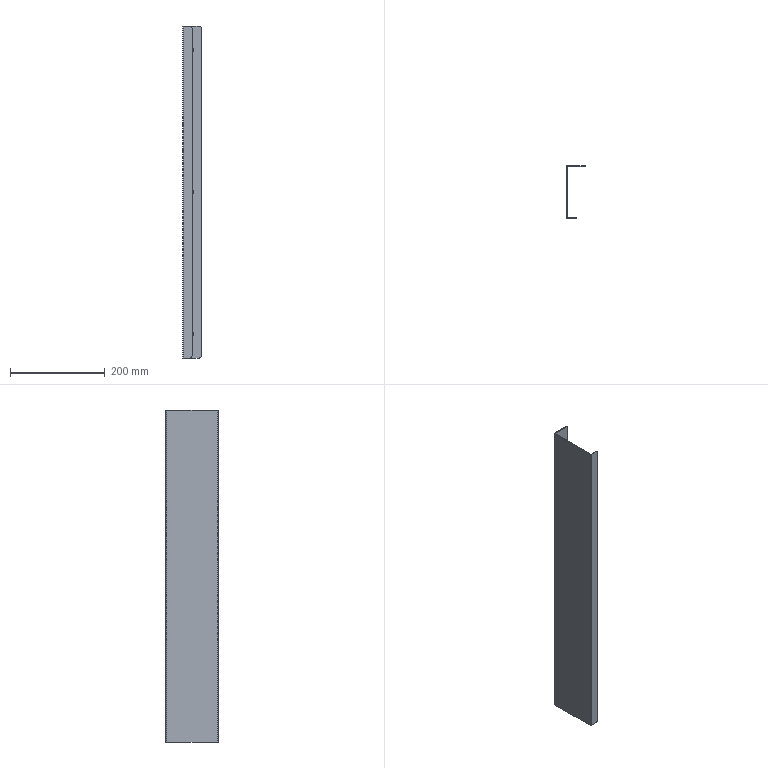Part | STEP file | HJDX-300 | 1 solid | 24 faces | box 40 x 110 x 700 mm | volume 173965 mm3 | cylinder 14 | plane 10 | commonest cylinder face diameters 8 x6 10 x4 1 x2 4 x2
STEP:
#1=CARTESIAN_POINT('',(22.5,53.5,-300.));
#2=VERTEX_POINT('',#1);
#3=CARTESIAN_POINT('',(14.5,53.5,-300.));
#4=VERTEX_POINT('',#3);
#5=CARTESIAN_POINT('',(18.5,53.5,-300.));
#6=DIRECTION('',(0.,1.,0.));
#7=DIRECTION('',(-1.,0.,0.));
#8=AXIS2_PLACEMENT_3D('',#5,#6,#7);
#9=CIRCLE('',#8,4.);
#10=EDGE_CURVE('',#2,#4,#9,.T.);
#11=ORIENTED_EDGE('',*,*,#10,.F.);
#12=CARTESIAN_POINT('',(22.5,55.,-300.));
#13=VERTEX_POINT('',#12);
#14=CARTESIAN_POINT('',(22.5,45.,-300.));
#15=DIRECTION('',(0.,1.,0.));
#16=VECTOR('',#15,1000.);
#17=LINE('',#14,#16);
#18=EDGE_CURVE('',#2,#13,#17,.T.);
#19=ORIENTED_EDGE('',*,*,#18,.T.);
#20=CARTESIAN_POINT('',(14.5,55.,-300.));
#21=VERTEX_POINT('',#20);
#22=CARTESIAN_POINT('',(18.5,55.,-300.));
#23=DIRECTION('',(0.,1.,0.));
#24=DIRECTION('',(-1.,0.,0.));
#25=AXIS2_PLACEMENT_3D('',#22,#23,#24);
#26=CIRCLE('',#25,4.);
#27=EDGE_CURVE('',#13,#21,#26,.T.);
#28=ORIENTED_EDGE('',*,*,#27,.T.);
#29=CARTESIAN_POINT('',(14.5,45.,-300.));
#30=DIRECTION('',(0.,1.,0.));
#31=VECTOR('',#30,1000.);
#32=LINE('',#29,#31);
#33=EDGE_CURVE('',#4,#21,#32,.T.);
#34=ORIENTED_EDGE('',*,*,#33,.F.);
#35=EDGE_LOOP('',(#11,#19,#28,#34));
#36=FACE_OUTER_BOUND('',#35,.T.);
#37=CARTESIAN_POINT('',(18.5,45.,-300.));
#38=DIRECTION('',(0.,1.,0.));
#39=DIRECTION('',(-1.,0.,0.));
#40=AXIS2_PLACEMENT_3D('',#37,#38,#39);
#41=CYLINDRICAL_SURFACE('',#40,4.);
#42=ADVANCED_FACE('',(#36),#41,.F.);
#43=CARTESIAN_POINT('',(22.5,53.5,300.));
#44=VERTEX_POINT('',#43);
#45=CARTESIAN_POINT('',(14.5,53.5,300.));
#46=VERTEX_POINT('',#45);
#47=CARTESIAN_POINT('',(18.5,53.5,300.));
#48=DIRECTION('',(0.,1.,0.));
#49=DIRECTION('',(-1.,0.,0.));
#50=AXIS2_PLACEMENT_3D('',#47,#48,#49);
#51=CIRCLE('',#50,4.);
#52=EDGE_CURVE('',#44,#46,#51,.T.);
#53=ORIENTED_EDGE('',*,*,#52,.F.);
#54=CARTESIAN_POINT('',(22.5,55.,300.));
#55=VERTEX_POINT('',#54);
#56=CARTESIAN_POINT('',(22.5,45.,300.));
#57=DIRECTION('',(0.,1.,0.));
#58=VECTOR('',#57,1000.);
#59=LINE('',#56,#58);
#60=EDGE_CURVE('',#44,#55,#59,.T.);
#61=ORIENTED_EDGE('',*,*,#60,.T.);
#62=CARTESIAN_POINT('',(14.5,55.,300.));
#63=VERTEX_POINT('',#62);
#64=CARTESIAN_POINT('',(18.5,55.,300.));
#65=DIRECTION('',(0.,1.,0.));
#66=DIRECTION('',(-1.,0.,0.));
#67=AXIS2_PLACEMENT_3D('',#64,#65,#66);
#68=CIRCLE('',#67,4.);
#69=EDGE_CURVE('',#55,#63,#68,.T.);
#70=ORIENTED_EDGE('',*,*,#69,.T.);
#71=CARTESIAN_POINT('',(14.5,45.,300.));
#72=DIRECTION('',(0.,1.,0.));
#73=VECTOR('',#72,1000.);
#74=LINE('',#71,#73);
#75=EDGE_CURVE('',#46,#63,#74,.T.);
#76=ORIENTED_EDGE('',*,*,#75,.F.);
#77=EDGE_LOOP('',(#53,#61,#70,#76));
#78=FACE_OUTER_BOUND('',#77,.T.);
#79=CARTESIAN_POINT('',(18.5,45.,300.));
#80=DIRECTION('',(0.,1.,0.));
#81=DIRECTION('',(-1.,0.,0.));
#82=AXIS2_PLACEMENT_3D('',#79,#80,#81);
#83=CYLINDRICAL_SURFACE('',#82,4.);
#84=ADVANCED_FACE('',(#78),#83,.F.);
#85=CARTESIAN_POINT('',(22.5,53.5,0.));
#86=VERTEX_POINT('',#85);
#87=CARTESIAN_POINT('',(14.5,53.5,0.));
#88=VERTEX_POINT('',#87);
#89=CARTESIAN_POINT('',(18.5,53.5,0.));
#90=DIRECTION('',(0.,1.,0.));
#91=DIRECTION('',(-1.,0.,0.));
#92=AXIS2_PLACEMENT_3D('',#89,#90,#91);
#93=CIRCLE('',#92,4.);
#94=EDGE_CURVE('',#86,#88,#93,.T.);
#95=ORIENTED_EDGE('',*,*,#94,.F.);
#96=CARTESIAN_POINT('',(22.5,55.,0.));
#97=VERTEX_POINT('',#96);
#98=CARTESIAN_POINT('',(22.5,45.,0.));
#99=DIRECTION('',(0.,1.,0.));
#100=VECTOR('',#99,1000.);
#101=LINE('',#98,#100);
#102=EDGE_CURVE('',#86,#97,#101,.T.);
#103=ORIENTED_EDGE('',*,*,#102,.T.);
#104=CARTESIAN_POINT('',(14.5,55.,0.));
#105=VERTEX_POINT('',#104);
#106=CARTESIAN_POINT('',(18.5,55.,0.));
#107=DIRECTION('',(0.,1.,0.));
#108=DIRECTION('',(-1.,0.,0.));
#109=AXIS2_PLACEMENT_3D('',#106,#107,#108);
#110=CIRCLE('',#109,4.);
#111=EDGE_CURVE('',#97,#105,#110,.T.);
#112=ORIENTED_EDGE('',*,*,#111,.T.);
#113=CARTESIAN_POINT('',(14.5,45.,0.));
#114=DIRECTION('',(0.,1.,0.));
#115=VECTOR('',#114,1000.);
#116=LINE('',#113,#115);
#117=EDGE_CURVE('',#88,#105,#116,.T.);
#118=ORIENTED_EDGE('',*,*,#117,.F.);
#119=EDGE_LOOP('',(#95,#103,#112,#118));
#120=FACE_OUTER_BOUND('',#119,.T.);
#121=CARTESIAN_POINT('',(18.5,45.,0.));
#122=DIRECTION('',(0.,1.,0.));
#123=DIRECTION('',(-1.,0.,0.));
#124=AXIS2_PLACEMENT_3D('',#121,#122,#123);
#125=CYLINDRICAL_SURFACE('',#124,4.);
#126=ADVANCED_FACE('',(#120),#125,.F.);
#127=CARTESIAN_POINT('',(-1.5,-53.,350.));
#128=VERTEX_POINT('',#127);
#129=CARTESIAN_POINT('',(-1.5,53.,350.));
#130=VERTEX_POINT('',#129);
#131=CARTESIAN_POINT('',(-1.5,0.,350.));
#132=DIRECTION('',(0.,1.,0.));
#133=VECTOR('',#132,1000.);
#134=LINE('',#131,#133);
#135=EDGE_CURVE('',#128,#130,#134,.T.);
#136=ORIENTED_EDGE('',*,*,#135,.T.);
#137=CARTESIAN_POINT('',(-1.5,53.,-350.));
#138=VERTEX_POINT('',#137);
#139=CARTESIAN_POINT('',(-1.5,53.,0.));
#140=DIRECTION('',(0.,0.,-1.));
#141=VECTOR('',#140,1000.);
#142=LINE('',#139,#141);
#143=EDGE_CURVE('',#130,#138,#142,.T.);
#144=ORIENTED_EDGE('',*,*,#143,.T.);
#145=CARTESIAN_POINT('',(-1.5,-53.,-350.));
#146=VERTEX_POINT('',#145);
#147=CARTESIAN_POINT('',(-1.5,0.,-350.));
#148=DIRECTION('',(0.,-1.,0.));
#149=VECTOR('',#148,1000.);
#150=LINE('',#147,#149);
#151=EDGE_CURVE('',#138,#146,#150,.T.);
#152=ORIENTED_EDGE('',*,*,#151,.T.);
#153=CARTESIAN_POINT('',(-1.5,-53.,0.));
#154=DIRECTION('',(0.,0.,1.));
#155=VECTOR('',#154,1000.);
#156=LINE('',#153,#155);
#157=EDGE_CURVE('',#146,#128,#156,.T.);
#158=ORIENTED_EDGE('',*,*,#157,.T.);
#159=EDGE_LOOP('',(#136,#144,#152,#158));
#160=FACE_OUTER_BOUND('',#159,.T.);
#161=CARTESIAN_POINT('',(-1.5,0.,0.));
#162=DIRECTION('',(-1.,0.,0.));
#163=DIRECTION('',(0.,0.,1.));
#164=AXIS2_PLACEMENT_3D('',#161,#162,#163);
#165=PLANE('',#164);
#166=ADVANCED_FACE('',(#160),#165,.T.);
#167=CARTESIAN_POINT('',(0.5,55.,350.));
#168=VERTEX_POINT('',#167);
#169=CARTESIAN_POINT('',(0.5,55.,-350.));
#170=VERTEX_POINT('',#169);
#171=CARTESIAN_POINT('',(0.5,55.,350.));
#172=DIRECTION('',(0.,0.,-1.));
#173=VECTOR('',#172,1000.);
#174=LINE('',#171,#173);
#175=EDGE_CURVE('',#168,#170,#174,.T.);
#176=ORIENTED_EDGE('',*,*,#175,.T.);
#177=CARTESIAN_POINT('',(0.5,53.,-350.));
#178=DIRECTION('',(0.,0.,1.));
#179=DIRECTION('',(1.,0.,0.));
#180=AXIS2_PLACEMENT_3D('',#177,#178,#179);
#181=CIRCLE('',#180,2.);
#182=EDGE_CURVE('',#170,#138,#181,.T.);
#183=ORIENTED_EDGE('',*,*,#182,.T.);
#184=ORIENTED_EDGE('',*,*,#143,.F.);
#185=CARTESIAN_POINT('',(0.5,53.,350.));
#186=DIRECTION('',(0.,0.,-1.));
#187=DIRECTION('',(1.,0.,0.));
#188=AXIS2_PLACEMENT_3D('',#185,#186,#187);
#189=CIRCLE('',#188,2.);
#190=EDGE_CURVE('',#130,#168,#189,.T.);
#191=ORIENTED_EDGE('',*,*,#190,.T.);
#192=EDGE_LOOP('',(#176,#183,#184,#191));
#193=FACE_OUTER_BOUND('',#192,.T.);
#194=CARTESIAN_POINT('',(0.5,53.,350.));
#195=DIRECTION('',(0.,0.,1.));
#196=DIRECTION('',(1.,0.,0.));
#197=AXIS2_PLACEMENT_3D('',#194,#195,#196);
#198=CYLINDRICAL_SURFACE('',#197,2.);
#199=ADVANCED_FACE('',(#193),#198,.T.);
#200=CARTESIAN_POINT('',(0.,-53.,350.));
#201=VERTEX_POINT('',#200);
#202=CARTESIAN_POINT('',(0.,53.,350.));
#203=VERTEX_POINT('',#202);
#204=CARTESIAN_POINT('',(0.,-55.,350.));
#205=DIRECTION('',(0.,1.,0.));
#206=VECTOR('',#205,1000.);
#207=LINE('',#204,#206);
#208=EDGE_CURVE('',#201,#203,#207,.T.);
#209=ORIENTED_EDGE('',*,*,#208,.T.);
#210=CARTESIAN_POINT('',(0.5,53.5,350.));
#211=VERTEX_POINT('',#210);
#212=CARTESIAN_POINT('',(0.5,53.,350.));
#213=DIRECTION('',(0.,0.,-1.));
#214=DIRECTION('',(1.,0.,0.));
#215=AXIS2_PLACEMENT_3D('',#212,#213,#214);
#216=CIRCLE('',#215,0.5);
#217=EDGE_CURVE('',#203,#211,#216,.T.);
#218=ORIENTED_EDGE('',*,*,#217,.T.);
#219=CARTESIAN_POINT('',(33.5,53.5,350.));
#220=VERTEX_POINT('',#219);
#221=CARTESIAN_POINT('',(38.5,53.5,350.));
#222=DIRECTION('',(-1.,0.,0.));
#223=VECTOR('',#222,1000.);
#224=LINE('',#221,#223);
#225=EDGE_CURVE('',#220,#211,#224,.T.);
#226=ORIENTED_EDGE('',*,*,#225,.F.);
#227=CARTESIAN_POINT('',(33.5,55.,350.));
#228=VERTEX_POINT('',#227);
#229=CARTESIAN_POINT('',(33.5,55.,350.));
#230=DIRECTION('',(0.,-1.,0.));
#231=VECTOR('',#230,1000.);
#232=LINE('',#229,#231);
#233=EDGE_CURVE('',#228,#220,#232,.T.);
#234=ORIENTED_EDGE('',*,*,#233,.F.);
#235=CARTESIAN_POINT('',(0.,55.,350.));
#236=DIRECTION('',(-1.,0.,0.));
#237=VECTOR('',#236,1000.);
#238=LINE('',#235,#237);
#239=EDGE_CURVE('',#228,#168,#238,.T.);
#240=ORIENTED_EDGE('',*,*,#239,.T.);
#241=ORIENTED_EDGE('',*,*,#190,.F.);
#242=ORIENTED_EDGE('',*,*,#135,.F.);
#243=CARTESIAN_POINT('',(0.5,-55.,350.));
#244=VERTEX_POINT('',#243);
#245=CARTESIAN_POINT('',(0.5,-53.,350.));
#246=DIRECTION('',(0.,0.,-1.));
#247=DIRECTION('',(-1.,0.,0.));
#248=AXIS2_PLACEMENT_3D('',#245,#246,#247);
#249=CIRCLE('',#248,2.);
#250=EDGE_CURVE('',#244,#128,#249,.T.);
#251=ORIENTED_EDGE('',*,*,#250,.F.);
#252=CARTESIAN_POINT('',(13.5,-55.,350.));
#253=VERTEX_POINT('',#252);
#254=CARTESIAN_POINT('',(0.,-55.,350.));
#255=DIRECTION('',(1.,0.,0.));
#256=VECTOR('',#255,1000.);
#257=LINE('',#254,#256);
#258=EDGE_CURVE('',#244,#253,#257,.T.);
#259=ORIENTED_EDGE('',*,*,#258,.T.);
#260=CARTESIAN_POINT('',(13.5,-53.5,350.));
#261=VERTEX_POINT('',#260);
#262=CARTESIAN_POINT('',(13.5,-55.,350.));
#263=DIRECTION('',(0.,-1.,0.));
#264=VECTOR('',#263,1000.);
#265=LINE('',#262,#264);
#266=EDGE_CURVE('',#261,#253,#265,.T.);
#267=ORIENTED_EDGE('',*,*,#266,.F.);
#268=CARTESIAN_POINT('',(0.5,-53.5,350.));
#269=VERTEX_POINT('',#268);
#270=CARTESIAN_POINT('',(0.,-53.5,350.));
#271=DIRECTION('',(1.,0.,0.));
#272=VECTOR('',#271,1000.);
#273=LINE('',#270,#272);
#274=EDGE_CURVE('',#269,#261,#273,.T.);
#275=ORIENTED_EDGE('',*,*,#274,.F.);
#276=CARTESIAN_POINT('',(0.5,-53.,350.));
#277=DIRECTION('',(0.,0.,-1.));
#278=DIRECTION('',(-1.,0.,0.));
#279=AXIS2_PLACEMENT_3D('',#276,#277,#278);
#280=CIRCLE('',#279,0.5);
#281=EDGE_CURVE('',#269,#201,#280,.T.);
#282=ORIENTED_EDGE('',*,*,#281,.T.);
#283=EDGE_LOOP('',(#209,#218,#226,#234,#240,#241,#242,#251,#259,#267,#275,#282));
#284=FACE_OUTER_BOUND('',#283,.T.);
#285=CARTESIAN_POINT('',(-1.5,-55.,350.));
#286=DIRECTION('',(0.,0.,1.));
#287=DIRECTION('',(1.,0.,0.));
#288=AXIS2_PLACEMENT_3D('',#285,#286,#287);
#289=PLANE('',#288);
#290=ADVANCED_FACE('',(#284),#289,.T.);
#291=CARTESIAN_POINT('',(0.5,-55.,-350.));
#292=VERTEX_POINT('',#291);
#293=CARTESIAN_POINT('',(0.5,-55.,-350.));
#294=DIRECTION('',(0.,0.,1.));
#295=VECTOR('',#294,1000.);
#296=LINE('',#293,#295);
#297=EDGE_CURVE('',#292,#244,#296,.T.);
#298=ORIENTED_EDGE('',*,*,#297,.T.);
#299=ORIENTED_EDGE('',*,*,#250,.T.);
#300=ORIENTED_EDGE('',*,*,#157,.F.);
#301=CARTESIAN_POINT('',(0.5,-53.,-350.));
#302=DIRECTION('',(0.,0.,1.));
#303=DIRECTION('',(-1.,0.,0.));
#304=AXIS2_PLACEMENT_3D('',#301,#302,#303);
#305=CIRCLE('',#304,2.);
#306=EDGE_CURVE('',#146,#292,#305,.T.);
#307=ORIENTED_EDGE('',*,*,#306,.T.);
#308=EDGE_LOOP('',(#298,#299,#300,#307));
#309=FACE_OUTER_BOUND('',#308,.T.);
#310=CARTESIAN_POINT('',(0.5,-53.,-350.));
#311=DIRECTION('',(0.,0.,-1.));
#312=DIRECTION('',(-1.,0.,0.));
#313=AXIS2_PLACEMENT_3D('',#310,#311,#312);
#314=CYLINDRICAL_SURFACE('',#313,2.);
#315=ADVANCED_FACE('',(#309),#314,.T.);
#316=ORIENTED_EDGE('',*,*,#151,.F.);
#317=ORIENTED_EDGE('',*,*,#182,.F.);
#318=CARTESIAN_POINT('',(33.5,55.,-350.));
#319=VERTEX_POINT('',#318);
#320=CARTESIAN_POINT('',(0.,55.,-350.));
#321=DIRECTION('',(1.,0.,0.));
#322=VECTOR('',#321,1000.);
#323=LINE('',#320,#322);
#324=EDGE_CURVE('',#170,#319,#323,.T.);
#325=ORIENTED_EDGE('',*,*,#324,.T.);
#326=CARTESIAN_POINT('',(33.5,53.5,-350.));
#327=VERTEX_POINT('',#326);
#328=CARTESIAN_POINT('',(33.5,55.,-350.));
#329=DIRECTION('',(0.,1.,0.));
#330=VECTOR('',#329,1000.);
#331=LINE('',#328,#330);
#332=EDGE_CURVE('',#327,#319,#331,.T.);
#333=ORIENTED_EDGE('',*,*,#332,.F.);
#334=CARTESIAN_POINT('',(0.5,53.5,-350.));
#335=VERTEX_POINT('',#334);
#336=CARTESIAN_POINT('',(0.,53.5,-350.));
#337=DIRECTION('',(1.,0.,0.));
#338=VECTOR('',#337,1000.);
#339=LINE('',#336,#338);
#340=EDGE_CURVE('',#335,#327,#339,.T.);
#341=ORIENTED_EDGE('',*,*,#340,.F.);
#342=CARTESIAN_POINT('',(0.,53.,-350.));
#343=VERTEX_POINT('',#342);
#344=CARTESIAN_POINT('',(0.5,53.,-350.));
#345=DIRECTION('',(0.,0.,1.));
#346=DIRECTION('',(1.,0.,0.));
#347=AXIS2_PLACEMENT_3D('',#344,#345,#346);
#348=CIRCLE('',#347,0.5);
#349=EDGE_CURVE('',#335,#343,#348,.T.);
#350=ORIENTED_EDGE('',*,*,#349,.T.);
#351=CARTESIAN_POINT('',(0.,-53.,-350.));
#352=VERTEX_POINT('',#351);
#353=CARTESIAN_POINT('',(0.,-55.,-350.));
#354=DIRECTION('',(0.,-1.,0.));
#355=VECTOR('',#354,1000.);
#356=LINE('',#353,#355);
#357=EDGE_CURVE('',#343,#352,#356,.T.);
#358=ORIENTED_EDGE('',*,*,#357,.T.);
#359=CARTESIAN_POINT('',(0.5,-53.5,-350.));
#360=VERTEX_POINT('',#359);
#361=CARTESIAN_POINT('',(0.5,-53.,-350.));
#362=DIRECTION('',(0.,0.,-1.));
#363=DIRECTION('',(-1.,0.,0.));
#364=AXIS2_PLACEMENT_3D('',#361,#362,#363);
#365=CIRCLE('',#364,0.5);
#366=EDGE_CURVE('',#360,#352,#365,.T.);
#367=ORIENTED_EDGE('',*,*,#366,.F.);
#368=CARTESIAN_POINT('',(13.5,-53.5,-350.));
#369=VERTEX_POINT('',#368);
#370=CARTESIAN_POINT('',(18.5,-53.5,-350.));
#371=DIRECTION('',(-1.,0.,0.));
#372=VECTOR('',#371,1000.);
#373=LINE('',#370,#372);
#374=EDGE_CURVE('',#369,#360,#373,.T.);
#375=ORIENTED_EDGE('',*,*,#374,.F.);
#376=CARTESIAN_POINT('',(13.5,-55.,-350.));
#377=VERTEX_POINT('',#376);
#378=CARTESIAN_POINT('',(13.5,-55.,-350.));
#379=DIRECTION('',(0.,1.,0.));
#380=VECTOR('',#379,1000.);
#381=LINE('',#378,#380);
#382=EDGE_CURVE('',#377,#369,#381,.T.);
#383=ORIENTED_EDGE('',*,*,#382,.F.);
#384=CARTESIAN_POINT('',(0.,-55.,-350.));
#385=DIRECTION('',(-1.,0.,0.));
#386=VECTOR('',#385,1000.);
#387=LINE('',#384,#386);
#388=EDGE_CURVE('',#377,#292,#387,.T.);
#389=ORIENTED_EDGE('',*,*,#388,.T.);
#390=ORIENTED_EDGE('',*,*,#306,.F.);
#391=EDGE_LOOP('',(#316,#317,#325,#333,#341,#350,#358,#367,#375,#383,#389,#390));
#392=FACE_OUTER_BOUND('',#391,.T.);
#393=CARTESIAN_POINT('',(-1.5,-55.,-350.));
#394=DIRECTION('',(0.,0.,-1.));
#395=DIRECTION('',(-1.,0.,0.));
#396=AXIS2_PLACEMENT_3D('',#393,#394,#395);
#397=PLANE('',#396);
#398=ADVANCED_FACE('',(#392),#397,.T.);
#399=CARTESIAN_POINT('',(18.5,55.,-300.));
#400=DIRECTION('',(0.,1.,0.));
#401=DIRECTION('',(-1.,0.,0.));
#402=AXIS2_PLACEMENT_3D('',#399,#400,#401);
#403=CIRCLE('',#402,4.);
#404=EDGE_CURVE('',#21,#13,#403,.T.);
#405=ORIENTED_EDGE('',*,*,#404,.F.);
#406=ORIENTED_EDGE('',*,*,#27,.F.);
#407=EDGE_LOOP('',(#405,#406));
#408=FACE_BOUND('',#407,.T.);
#409=CARTESIAN_POINT('',(38.5,55.,-345.));
#410=VERTEX_POINT('',#409);
#411=CARTESIAN_POINT('',(33.5,55.,-345.));
#412=DIRECTION('',(0.,-1.,0.));
#413=DIRECTION('',(1.,0.,0.));
#414=AXIS2_PLACEMENT_3D('',#411,#412,#413);
#415=CIRCLE('',#414,5.);
#416=EDGE_CURVE('',#319,#410,#415,.T.);
#417=ORIENTED_EDGE('',*,*,#416,.F.);
#418=ORIENTED_EDGE('',*,*,#324,.F.);
#419=ORIENTED_EDGE('',*,*,#175,.F.);
#420=ORIENTED_EDGE('',*,*,#239,.F.);
#421=CARTESIAN_POINT('',(38.5,55.,345.));
#422=VERTEX_POINT('',#421);
#423=CARTESIAN_POINT('',(33.5,55.,345.));
#424=DIRECTION('',(0.,-1.,0.));
#425=DIRECTION('',(1.,0.,0.));
#426=AXIS2_PLACEMENT_3D('',#423,#424,#425);
#427=CIRCLE('',#426,5.);
#428=EDGE_CURVE('',#422,#228,#427,.T.);
#429=ORIENTED_EDGE('',*,*,#428,.F.);
#430=CARTESIAN_POINT('',(38.5,55.,0.));
#431=DIRECTION('',(0.,0.,1.));
#432=VECTOR('',#431,1000.);
#433=LINE('',#430,#432);
#434=EDGE_CURVE('',#410,#422,#433,.T.);
#435=ORIENTED_EDGE('',*,*,#434,.F.);
#436=EDGE_LOOP('',(#417,#418,#419,#420,#429,#435));
#437=FACE_OUTER_BOUND('',#436,.T.);
#438=CARTESIAN_POINT('',(18.5,55.,300.));
#439=DIRECTION('',(0.,1.,0.));
#440=DIRECTION('',(-1.,0.,0.));
#441=AXIS2_PLACEMENT_3D('',#438,#439,#440);
#442=CIRCLE('',#441,4.);
#443=EDGE_CURVE('',#63,#55,#442,.T.);
#444=ORIENTED_EDGE('',*,*,#443,.F.);
#445=ORIENTED_EDGE('',*,*,#69,.F.);
#446=EDGE_LOOP('',(#444,#445));
#447=FACE_BOUND('',#446,.T.);
#448=CARTESIAN_POINT('',(18.5,55.,0.));
#449=DIRECTION('',(0.,1.,0.));
#450=DIRECTION('',(-1.,0.,0.));
#451=AXIS2_PLACEMENT_3D('',#448,#449,#450);
#452=CIRCLE('',#451,4.);
#453=EDGE_CURVE('',#105,#97,#452,.T.);
#454=ORIENTED_EDGE('',*,*,#453,.F.);
#455=ORIENTED_EDGE('',*,*,#111,.F.);
#456=EDGE_LOOP('',(#454,#455));
#457=FACE_BOUND('',#456,.T.);
#458=CARTESIAN_POINT('',(0.,55.,0.));
#459=DIRECTION('',(0.,-1.,0.));
#460=DIRECTION('',(1.,0.,0.));
#461=AXIS2_PLACEMENT_3D('',#458,#459,#460);
#462=PLANE('',#461);
#463=ADVANCED_FACE('',(#408,#437,#447,#457),#462,.F.);
#464=ORIENTED_EDGE('',*,*,#357,.F.);
#465=CARTESIAN_POINT('',(0.,53.,0.));
#466=DIRECTION('',(0.,0.,-1.));
#467=VECTOR('',#466,1000.);
#468=LINE('',#465,#467);
#469=EDGE_CURVE('',#203,#343,#468,.T.);
#470=ORIENTED_EDGE('',*,*,#469,.F.);
#471=ORIENTED_EDGE('',*,*,#208,.F.);
#472=CARTESIAN_POINT('',(0.,-53.,0.));
#473=DIRECTION('',(0.,0.,1.));
#474=VECTOR('',#473,1000.);
#475=LINE('',#472,#474);
#476=EDGE_CURVE('',#352,#201,#475,.T.);
#477=ORIENTED_EDGE('',*,*,#476,.F.);
#478=EDGE_LOOP('',(#464,#470,#471,#477));
#479=FACE_OUTER_BOUND('',#478,.T.);
#480=CARTESIAN_POINT('',(0.,0.,0.));
#481=DIRECTION('',(-1.,0.,0.));
#482=DIRECTION('',(0.,0.,1.));
#483=AXIS2_PLACEMENT_3D('',#480,#481,#482);
#484=PLANE('',#483);
#485=ADVANCED_FACE('',(#479),#484,.F.);
#486=CARTESIAN_POINT('',(18.5,-55.,-345.));
#487=VERTEX_POINT('',#486);
#488=CARTESIAN_POINT('',(13.5,-55.,-345.));
#489=DIRECTION('',(0.,1.,0.));
#490=DIRECTION('',(-1.,0.,0.));
#491=AXIS2_PLACEMENT_3D('',#488,#489,#490);
#492=CIRCLE('',#491,5.);
#493=EDGE_CURVE('',#487,#377,#492,.T.);
#494=ORIENTED_EDGE('',*,*,#493,.F.);
#495=CARTESIAN_POINT('',(18.5,-55.,345.));
#496=VERTEX_POINT('',#495);
#497=CARTESIAN_POINT('',(18.5,-55.,0.));
#498=DIRECTION('',(0.,0.,-1.));
#499=VECTOR('',#498,1000.);
#500=LINE('',#497,#499);
#501=EDGE_CURVE('',#496,#487,#500,.T.);
#502=ORIENTED_EDGE('',*,*,#501,.F.);
#503=CARTESIAN_POINT('',(13.5,-55.,345.));
#504=DIRECTION('',(0.,1.,0.));
#505=DIRECTION('',(-1.,0.,0.));
#506=AXIS2_PLACEMENT_3D('',#503,#504,#505);
#507=CIRCLE('',#506,5.);
#508=EDGE_CURVE('',#253,#496,#507,.T.);
#509=ORIENTED_EDGE('',*,*,#508,.F.);
#510=ORIENTED_EDGE('',*,*,#258,.F.);
#511=ORIENTED_EDGE('',*,*,#297,.F.);
#512=ORIENTED_EDGE('',*,*,#388,.F.);
#513=EDGE_LOOP('',(#494,#502,#509,#510,#511,#512));
#514=FACE_OUTER_BOUND('',#513,.T.);
#515=CARTESIAN_POINT('',(0.,-55.,0.));
#516=DIRECTION('',(0.,1.,0.));
#517=DIRECTION('',(-1.,0.,0.));
#518=AXIS2_PLACEMENT_3D('',#515,#516,#517);
#519=PLANE('',#518);
#520=ADVANCED_FACE('',(#514),#519,.F.);
#521=ORIENTED_EDGE('',*,*,#18,.F.);
#522=CARTESIAN_POINT('',(18.5,53.5,-300.));
#523=DIRECTION('',(0.,1.,0.));
#524=DIRECTION('',(-1.,0.,0.));
#525=AXIS2_PLACEMENT_3D('',#522,#523,#524);
#526=CIRCLE('',#525,4.);
#527=EDGE_CURVE('',#4,#2,#526,.T.);
#528=ORIENTED_EDGE('',*,*,#527,.F.);
#529=ORIENTED_EDGE('',*,*,#33,.T.);
#530=ORIENTED_EDGE('',*,*,#404,.T.);
#531=EDGE_LOOP('',(#521,#528,#529,#530));
#532=FACE_OUTER_BOUND('',#531,.T.);
#533=CARTESIAN_POINT('',(18.5,45.,-300.));
#534=DIRECTION('',(0.,1.,0.));
#535=DIRECTION('',(-1.,0.,0.));
#536=AXIS2_PLACEMENT_3D('',#533,#534,#535);
#537=CYLINDRICAL_SURFACE('',#536,4.);
#538=ADVANCED_FACE('',(#532),#537,.F.);
#539=CARTESIAN_POINT('',(38.5,53.5,-345.));
#540=VERTEX_POINT('',#539);
#541=CARTESIAN_POINT('',(38.5,55.,-345.));
#542=DIRECTION('',(0.,-1.,0.));
#543=VECTOR('',#542,1000.);
#544=LINE('',#541,#543);
#545=EDGE_CURVE('',#410,#540,#544,.T.);
#546=ORIENTED_EDGE('',*,*,#545,.F.);
#547=ORIENTED_EDGE('',*,*,#434,.T.);
#548=CARTESIAN_POINT('',(38.5,53.5,345.));
#549=VERTEX_POINT('',#548);
#550=CARTESIAN_POINT('',(38.5,55.,345.));
#551=DIRECTION('',(0.,1.,0.));
#552=VECTOR('',#551,1000.);
#553=LINE('',#550,#552);
#554=EDGE_CURVE('',#549,#422,#553,.T.);
#555=ORIENTED_EDGE('',*,*,#554,.F.);
#556=CARTESIAN_POINT('',(38.5,53.5,-350.));
#557=DIRECTION('',(0.,0.,1.));
#558=VECTOR('',#557,1000.);
#559=LINE('',#556,#558);
#560=EDGE_CURVE('',#540,#549,#559,.T.);
#561=ORIENTED_EDGE('',*,*,#560,.F.);
#562=EDGE_LOOP('',(#546,#547,#555,#561));
#563=FACE_OUTER_BOUND('',#562,.T.);
#564=CARTESIAN_POINT('',(38.5,55.,-350.));
#565=DIRECTION('',(-1.,0.,0.));
#566=DIRECTION('',(0.,-1.,0.));
#567=AXIS2_PLACEMENT_3D('',#564,#565,#566);
#568=PLANE('',#567);
#569=ADVANCED_FACE('',(#563),#568,.F.);
#570=CARTESIAN_POINT('',(33.5,53.5,-345.));
#571=DIRECTION('',(0.,1.,0.));
#572=DIRECTION('',(1.,0.,0.));
#573=AXIS2_PLACEMENT_3D('',#570,#571,#572);
#574=CIRCLE('',#573,5.);
#575=EDGE_CURVE('',#540,#327,#574,.T.);
#576=ORIENTED_EDGE('',*,*,#575,.T.);
#577=ORIENTED_EDGE('',*,*,#332,.T.);
#578=ORIENTED_EDGE('',*,*,#416,.T.);
#579=ORIENTED_EDGE('',*,*,#545,.T.);
#580=EDGE_LOOP('',(#576,#577,#578,#579));
#581=FACE_OUTER_BOUND('',#580,.T.);
#582=CARTESIAN_POINT('',(33.5,55.,-345.));
#583=DIRECTION('',(0.,-1.,0.));
#584=DIRECTION('',(1.,0.,0.));
#585=AXIS2_PLACEMENT_3D('',#582,#583,#584);
#586=CYLINDRICAL_SURFACE('',#585,5.);
#587=ADVANCED_FACE('',(#581),#586,.T.);
#588=CARTESIAN_POINT('',(33.5,53.5,345.));
#589=DIRECTION('',(0.,1.,0.));
#590=DIRECTION('',(1.,0.,0.));
#591=AXIS2_PLACEMENT_3D('',#588,#589,#590);
#592=CIRCLE('',#591,5.);
#593=EDGE_CURVE('',#220,#549,#592,.T.);
#594=ORIENTED_EDGE('',*,*,#593,.T.);
#595=ORIENTED_EDGE('',*,*,#554,.T.);
#596=ORIENTED_EDGE('',*,*,#428,.T.);
#597=ORIENTED_EDGE('',*,*,#233,.T.);
#598=EDGE_LOOP('',(#594,#595,#596,#597));
#599=FACE_OUTER_BOUND('',#598,.T.);
#600=CARTESIAN_POINT('',(33.5,55.,345.));
#601=DIRECTION('',(0.,-1.,0.));
#602=DIRECTION('',(1.,0.,0.));
#603=AXIS2_PLACEMENT_3D('',#600,#601,#602);
#604=CYLINDRICAL_SURFACE('',#603,5.);
#605=ADVANCED_FACE('',(#599),#604,.T.);
#606=ORIENTED_EDGE('',*,*,#60,.F.);
#607=CARTESIAN_POINT('',(18.5,53.5,300.));
#608=DIRECTION('',(0.,1.,0.));
#609=DIRECTION('',(-1.,0.,0.));
#610=AXIS2_PLACEMENT_3D('',#607,#608,#609);
#611=CIRCLE('',#610,4.);
#612=EDGE_CURVE('',#46,#44,#611,.T.);
#613=ORIENTED_EDGE('',*,*,#612,.F.);
#614=ORIENTED_EDGE('',*,*,#75,.T.);
#615=ORIENTED_EDGE('',*,*,#443,.T.);
#616=EDGE_LOOP('',(#606,#613,#614,#615));
#617=FACE_OUTER_BOUND('',#616,.T.);
#618=CARTESIAN_POINT('',(18.5,45.,300.));
#619=DIRECTION('',(0.,1.,0.));
#620=DIRECTION('',(-1.,0.,0.));
#621=AXIS2_PLACEMENT_3D('',#618,#619,#620);
#622=CYLINDRICAL_SURFACE('',#621,4.);
#623=ADVANCED_FACE('',(#617),#622,.F.);
#624=ORIENTED_EDGE('',*,*,#102,.F.);
#625=CARTESIAN_POINT('',(18.5,53.5,0.));
#626=DIRECTION('',(0.,1.,0.));
#627=DIRECTION('',(-1.,0.,0.));
#628=AXIS2_PLACEMENT_3D('',#625,#626,#627);
#629=CIRCLE('',#628,4.);
#630=EDGE_CURVE('',#88,#86,#629,.T.);
#631=ORIENTED_EDGE('',*,*,#630,.F.);
#632=ORIENTED_EDGE('',*,*,#117,.T.);
#633=ORIENTED_EDGE('',*,*,#453,.T.);
#634=EDGE_LOOP('',(#624,#631,#632,#633));
#635=FACE_OUTER_BOUND('',#634,.T.);
#636=CARTESIAN_POINT('',(18.5,45.,0.));
#637=DIRECTION('',(0.,1.,0.));
#638=DIRECTION('',(-1.,0.,0.));
#639=AXIS2_PLACEMENT_3D('',#636,#637,#638);
#640=CYLINDRICAL_SURFACE('',#639,4.);
#641=ADVANCED_FACE('',(#635),#640,.F.);
#642=ORIENTED_EDGE('',*,*,#281,.F.);
#643=CARTESIAN_POINT('',(0.5,-53.5,-350.));
#644=DIRECTION('',(0.,0.,1.));
#645=VECTOR('',#644,1000.);
#646=LINE('',#643,#645);
#647=EDGE_CURVE('',#360,#269,#646,.T.);
#648=ORIENTED_EDGE('',*,*,#647,.F.);
#649=ORIENTED_EDGE('',*,*,#366,.T.);
#650=ORIENTED_EDGE('',*,*,#476,.T.);
#651=EDGE_LOOP('',(#642,#648,#649,#650));
#652=FACE_OUTER_BOUND('',#651,.T.);
#653=CARTESIAN_POINT('',(0.5,-53.,-350.));
#654=DIRECTION('',(0.,0.,-1.));
#655=DIRECTION('',(-1.,0.,0.));
#656=AXIS2_PLACEMENT_3D('',#653,#654,#655);
#657=CYLINDRICAL_SURFACE('',#656,0.5);
#658=ADVANCED_FACE('',(#652),#657,.F.);
#659=ORIENTED_EDGE('',*,*,#349,.F.);
#660=CARTESIAN_POINT('',(0.5,53.5,350.));
#661=DIRECTION('',(0.,0.,-1.));
#662=VECTOR('',#661,1000.);
#663=LINE('',#660,#662);
#664=EDGE_CURVE('',#211,#335,#663,.T.);
#665=ORIENTED_EDGE('',*,*,#664,.F.);
#666=ORIENTED_EDGE('',*,*,#217,.F.);
#667=ORIENTED_EDGE('',*,*,#469,.T.);
#668=EDGE_LOOP('',(#659,#665,#666,#667));
#669=FACE_OUTER_BOUND('',#668,.T.);
#670=CARTESIAN_POINT('',(0.5,53.,350.));
#671=DIRECTION('',(0.,0.,1.));
#672=DIRECTION('',(1.,0.,0.));
#673=AXIS2_PLACEMENT_3D('',#670,#671,#672);
#674=CYLINDRICAL_SURFACE('',#673,0.5);
#675=ADVANCED_FACE('',(#669),#674,.F.);
#676=CARTESIAN_POINT('',(18.5,-53.5,-345.));
#677=VERTEX_POINT('',#676);
#678=CARTESIAN_POINT('',(13.5,-53.5,-345.));
#679=DIRECTION('',(0.,-1.,0.));
#680=DIRECTION('',(-1.,0.,0.));
#681=AXIS2_PLACEMENT_3D('',#678,#679,#680);
#682=CIRCLE('',#681,5.);
#683=EDGE_CURVE('',#369,#677,#682,.T.);
#684=ORIENTED_EDGE('',*,*,#683,.T.);
#685=CARTESIAN_POINT('',(18.5,-55.,-345.));
#686=DIRECTION('',(0.,-1.,0.));
#687=VECTOR('',#686,1000.);
#688=LINE('',#685,#687);
#689=EDGE_CURVE('',#677,#487,#688,.T.);
#690=ORIENTED_EDGE('',*,*,#689,.T.);
#691=ORIENTED_EDGE('',*,*,#493,.T.);
#692=ORIENTED_EDGE('',*,*,#382,.T.);
#693=EDGE_LOOP('',(#684,#690,#691,#692));
#694=FACE_OUTER_BOUND('',#693,.T.);
#695=CARTESIAN_POINT('',(13.5,-55.,-345.));
#696=DIRECTION('',(0.,1.,0.));
#697=DIRECTION('',(-1.,0.,0.));
#698=AXIS2_PLACEMENT_3D('',#695,#696,#697);
#699=CYLINDRICAL_SURFACE('',#698,5.);
#700=ADVANCED_FACE('',(#694),#699,.T.);
#701=ORIENTED_EDGE('',*,*,#689,.F.);
#702=CARTESIAN_POINT('',(18.5,-53.5,345.));
#703=VERTEX_POINT('',#702);
#704=CARTESIAN_POINT('',(18.5,-53.5,350.));
#705=DIRECTION('',(0.,0.,-1.));
#706=VECTOR('',#705,1000.);
#707=LINE('',#704,#706);
#708=EDGE_CURVE('',#703,#677,#707,.T.);
#709=ORIENTED_EDGE('',*,*,#708,.F.);
#710=CARTESIAN_POINT('',(18.5,-55.,345.));
#711=DIRECTION('',(0.,1.,0.));
#712=VECTOR('',#711,1000.);
#713=LINE('',#710,#712);
#714=EDGE_CURVE('',#496,#703,#713,.T.);
#715=ORIENTED_EDGE('',*,*,#714,.F.);
#716=ORIENTED_EDGE('',*,*,#501,.T.);
#717=EDGE_LOOP('',(#701,#709,#715,#716));
#718=FACE_OUTER_BOUND('',#717,.T.);
#719=CARTESIAN_POINT('',(18.5,-55.,350.));
#720=DIRECTION('',(-1.,0.,0.));
#721=DIRECTION('',(0.,-1.,0.));
#722=AXIS2_PLACEMENT_3D('',#719,#720,#721);
#723=PLANE('',#722);
#724=ADVANCED_FACE('',(#718),#723,.F.);
#725=CARTESIAN_POINT('',(13.5,-53.5,345.));
#726=DIRECTION('',(0.,-1.,0.));
#727=DIRECTION('',(-1.,0.,0.));
#728=AXIS2_PLACEMENT_3D('',#725,#726,#727);
#729=CIRCLE('',#728,5.);
#730=EDGE_CURVE('',#703,#261,#729,.T.);
#731=ORIENTED_EDGE('',*,*,#730,.T.);
#732=ORIENTED_EDGE('',*,*,#266,.T.);
#733=ORIENTED_EDGE('',*,*,#508,.T.);
#734=ORIENTED_EDGE('',*,*,#714,.T.);
#735=EDGE_LOOP('',(#731,#732,#733,#734));
#736=FACE_OUTER_BOUND('',#735,.T.);
#737=CARTESIAN_POINT('',(13.5,-55.,345.));
#738=DIRECTION('',(0.,1.,0.));
#739=DIRECTION('',(-1.,0.,0.));
#740=AXIS2_PLACEMENT_3D('',#737,#738,#739);
#741=CYLINDRICAL_SURFACE('',#740,5.);
#742=ADVANCED_FACE('',(#736),#741,.T.);
#743=ORIENTED_EDGE('',*,*,#527,.T.);
#744=ORIENTED_EDGE('',*,*,#10,.T.);
#745=EDGE_LOOP('',(#743,#744));
#746=FACE_BOUND('',#745,.T.);
#747=ORIENTED_EDGE('',*,*,#225,.T.);
#748=ORIENTED_EDGE('',*,*,#664,.T.);
#749=ORIENTED_EDGE('',*,*,#340,.T.);
#750=ORIENTED_EDGE('',*,*,#575,.F.);
#751=ORIENTED_EDGE('',*,*,#560,.T.);
#752=ORIENTED_EDGE('',*,*,#593,.F.);
#753=EDGE_LOOP('',(#747,#748,#749,#750,#751,#752));
#754=FACE_OUTER_BOUND('',#753,.T.);
#755=ORIENTED_EDGE('',*,*,#612,.T.);
#756=ORIENTED_EDGE('',*,*,#52,.T.);
#757=EDGE_LOOP('',(#755,#756));
#758=FACE_BOUND('',#757,.T.);
#759=ORIENTED_EDGE('',*,*,#630,.T.);
#760=ORIENTED_EDGE('',*,*,#94,.T.);
#761=EDGE_LOOP('',(#759,#760));
#762=FACE_BOUND('',#761,.T.);
#763=CARTESIAN_POINT('',(0.,53.5,0.));
#764=DIRECTION('',(0.,-1.,0.));
#765=DIRECTION('',(1.,0.,0.));
#766=AXIS2_PLACEMENT_3D('',#763,#764,#765);
#767=PLANE('',#766);
#768=ADVANCED_FACE('',(#746,#754,#758,#762),#767,.T.);
#769=ORIENTED_EDGE('',*,*,#274,.T.);
#770=ORIENTED_EDGE('',*,*,#730,.F.);
#771=ORIENTED_EDGE('',*,*,#708,.T.);
#772=ORIENTED_EDGE('',*,*,#683,.F.);
#773=ORIENTED_EDGE('',*,*,#374,.T.);
#774=ORIENTED_EDGE('',*,*,#647,.T.);
#775=EDGE_LOOP('',(#769,#770,#771,#772,#773,#774));
#776=FACE_OUTER_BOUND('',#775,.T.);
#777=CARTESIAN_POINT('',(0.,-53.5,0.));
#778=DIRECTION('',(0.,1.,0.));
#779=DIRECTION('',(-1.,0.,0.));
#780=AXIS2_PLACEMENT_3D('',#777,#778,#779);
#781=PLANE('',#780);
#782=ADVANCED_FACE('',(#776),#781,.T.);
#783=CLOSED_SHELL('',(#42,#84,#126,#166,#199,#290,#315,#398,#463,#485,#520,#538,#569,#587,#605,#623,#641,#658,#675,#700,#724,#742,#768,#782));
#784=MANIFOLD_SOLID_BREP('',#783);
#785=CARTESIAN_POINT('',(0.,0.,0.));
#786=DIRECTION('',(0.,0.,1.));
#787=DIRECTION('',(1.,0.,0.));
#788=AXIS2_PLACEMENT_3D('',#785,#786,#787);
#789=(LENGTH_UNIT()NAMED_UNIT(*)SI_UNIT(.MILLI.,.METRE.));
#790=UNCERTAINTY_MEASURE_WITH_UNIT(LENGTH_MEASURE(0.00001),#789,'','');
#791=(NAMED_UNIT(*)PLANE_ANGLE_UNIT()SI_UNIT($,.RADIAN.));
#792=(NAMED_UNIT(*)SI_UNIT($,.STERADIAN.)SOLID_ANGLE_UNIT());
#793=(GEOMETRIC_REPRESENTATION_CONTEXT(3)GLOBAL_UNCERTAINTY_ASSIGNED_CONTEXT((#790))GLOBAL_UNIT_ASSIGNED_CONTEXT((#789,#791,#792))REPRESENTATION_CONTEXT('',''));
#794=ADVANCED_BREP_SHAPE_REPRESENTATION('',(#784,#788),#793);